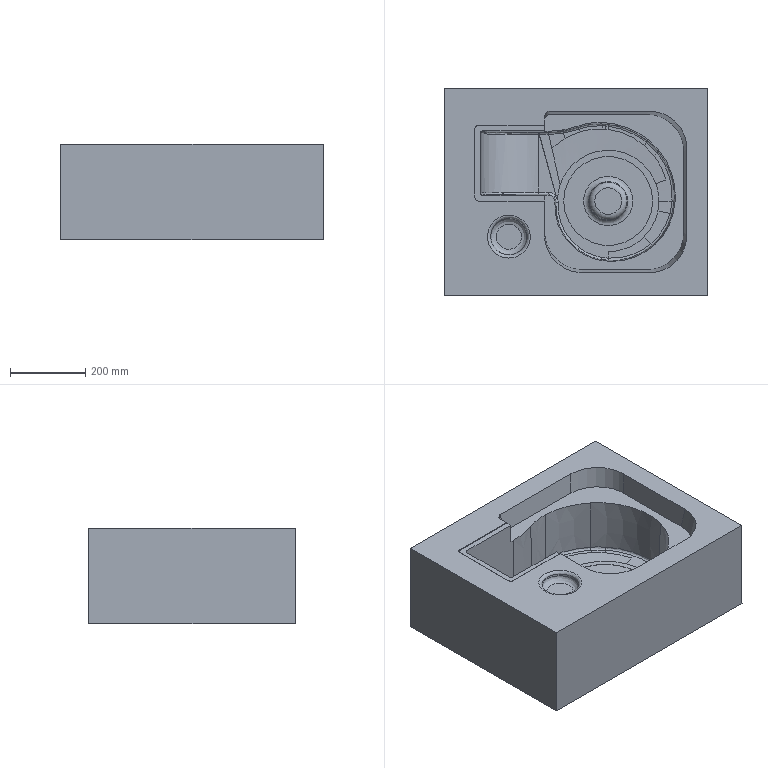NC program | NX | posted with a generic post | part box 700 x 550 x 255 mm
Lines 27406 to 28276 of 43405:
(ZLEVEL_PROFILE , TOOL : 20)
N54798 M6
N54800 G54
N54802 G17 G0 G90 X73.514 Y194.926 S2200 M3
N54804 G43 Z30. H0
N54806 Z0.47
N54808 G94 G1 Z-0.53 F2000.
N54810 G3 X63.514 Y204.926 R10.
N54812 G1 X-68.816
N54814 G3 X-72.579 Y203.186 R4.937
N54816 X-73.824 Y199.761 R5.246
N54818 G1 Y177.182
N54820 G2 X-83.823 Y167.182 R10.
N54822 G1 X-259.307
N54824 G3 X-259.902 Y166.586 R0.595
N54826 G1 Y-13.614
N54828 G3 X-259.307 Y-14.209 R0.595
N54830 G1 X-83.823
N54832 G2 X-73.824 Y-24.209 R10.
N54834 G1 Y-114.065
N54836 G3 X-57.772 Y-165.899 R91.581
N54838 X-18.435 Y-197.973 R90.032
N54840 X16.059 Y-204.926 R89.145
N54842 G1 X195.844
N54844 G3 X233.216 Y-196.836 R89.813
N54846 X279.873 Y-145.675 R88.255
N54848 X284.926 Y-115.894 R90.057
N54850 G1 Y115.894
N54852 G3 X276.844 Y153.199 R89.809
N54854 X226.261 Y199.665 R88.261
N54856 X195.844 Y204.926 R90.036
N54858 G1 X63.514
N54860 G3 X53.514 Y194.926 R10.
N54862 G1 Z0.47
N54864 G0 Z30.
N54866 X73.514 Y194.851
N54868 Z-0.06
N54870 G1 Z-1.06
N54872 G3 X63.514 Y204.851 R10.
N54874 G1 X-68.802
N54876 G3 X-72.812 Y202.812 R4.947
N54878 X-73.819 Y199.722 R5.27
N54880 G1 Y177.177
N54882 G2 X-83.819 Y167.177 R10.
N54884 G1 X-259.307
N54886 G3 X-259.898 Y166.586 R0.591
N54888 G1 Y-13.614
N54890 G3 X-259.307 Y-14.204 R0.591
N54892 G1 X-83.819
N54894 G2 X-73.819 Y-24.204 R10.
N54896 G1 Y-113.991
N54898 G3 X-57.277 Y-166.531 R91.583
N54900 X-17.171 Y-198.417 R90.01
N54902 X16.063 Y-204.851 R89.152
N54904 G1 X195.759
N54906 G3 X232.912 Y-196.866 R89.83
N54908 X280.006 Y-145.002 R88.261
N54910 X284.851 Y-115.816 R90.083
N54912 G1 Y115.816
N54914 G3 X276.995 Y152.627 R89.825
N54916 X224.996 Y200.008 R88.261
N54918 X195.759 Y204.851 R90.09
N54920 G1 X63.514
N54922 G3 X53.514 Y194.851 R10.
N54924 G1 Z-0.06
N54926 G0 Z30.
N54928 X73.514 Y194.777
N54930 Z-0.59
N54932 G1 Z-1.59
N54934 G3 X63.514 Y204.777 R10.
N54936 G1 X-68.787
N54938 G3 X-72.496 Y203.121 R4.929
N54940 X-73.814 Y199.588 R5.239
N54942 G1 Y177.173
N54944 G2 X-83.814 Y167.173 R10.
N54946 G1 X-259.307
N54948 G3 X-259.893 Y166.586 R0.586
N54950 G1 Y-13.614
N54952 G3 X-259.307 Y-14.2 R0.586
N54954 G1 X-83.814
N54956 G2 X-73.814 Y-24.2 R10.
N54958 G1 Y-113.916
N54960 G3 X-58.092 Y-165.267 R91.596
N54962 X-18.435 Y-197.82 R90.043
N54964 X16.068 Y-204.777 R89.148
N54966 G1 X195.683
N54968 G3 X231.952 Y-197.188 R89.86
N54970 X279.892 Y-145.043 R88.268
N54972 X284.777 Y-115.737 R90.098
N54974 G1 Y115.737
N54976 G3 X277.169 Y151.995 R89.847
N54978 X224.996 Y199.908 R88.271
N54980 X195.683 Y204.777 R90.107
N54982 G1 X63.514
N54984 G3 X53.514 Y194.777 R10.
N54986 G1 Z-0.59
N54988 G0 Z30.
N54990 X73.514 Y194.702
N54992 Z-1.12
N54994 G1 Z-2.12
N54996 G3 X63.514 Y204.702 R10.
N54998 G1 X-68.773
N55000 G3 X-72.812 Y202.651 R4.947
N55002 X-73.81 Y199.573 R5.271
N55004 G1 Y177.168
N55006 G2 X-83.81 Y167.168 R10.
N55008 G1 X-259.307
N55010 G3 X-259.889 Y166.586 R0.582
N55012 G1 Y-13.614
N55014 G3 X-259.307 Y-14.195 R0.582
N55016 G1 X-83.81
N55018 G2 X-73.81 Y-24.195 R10.
N55020 G1 Y-113.842
N55022 G3 X-59.291 Y-163.371 R91.639
N55024 X-24.126 Y-195.115 R90.185
N55026 X16.073 Y-204.702 R89.168
N55028 G1 X195.612
N55030 G3 X231.952 Y-197.081 R89.862
N55032 X279.792 Y-145.043 R88.266
N55034 X284.702 Y-115.658 R90.109
N55036 G1 Y115.658
N55038 G3 X276.779 Y152.627 R89.838
N55040 X224.996 Y199.808 R88.268
N55042 X195.612 Y204.702 R90.119
N55044 G1 X63.514
N55046 G3 X53.514 Y194.702 R10.
N55048 G1 Z-1.12
N55050 G0 Z30.
N55052 X-66.304 Y-0.066
N55054 Z-1.817
N55056 G1 Z-2.817
N55058 G3 X-73.804 Y-9.748 R10.
N55060 G1 Y-113.744
N55062 G3 X-58.902 Y-163.861 R91.634
N55064 X-22.861 Y-195.64 R90.139
N55066 X16.079 Y-204.604 R89.171
N55068 G1 X195.523
N55070 G3 X231.952 Y-196.939 R89.888
N55072 X279.659 Y-145.043 R88.267
N55074 X284.604 Y-115.554 R90.12
N55076 G1 Y115.554
N55078 G3 X277.197 Y151.363 R89.907
N55080 X224.996 Y199.675 R88.267
N55082 X195.523 Y204.604 R90.123
N55084 G1 X-68.753
N55086 G3 X-72.534 Y202.892 R4.927
N55088 X-73.796 Y199.647 R5.221
N55090 G1 X-73.804 Y199.394
N55092 Y162.721
N55094 G3 X-66.304 Y153.039 R10.
N55096 G1 Z-1.817
N55098 G0 Z30.
N55100 X-66.297 Y-0.054
N55102 Z-2.515
N55104 G1 Z-3.515
N55106 G3 X-73.797 Y-9.736 R10.
N55108 G1 Y-113.646
N55110 G3 X-59.151 Y-163.371 R91.655
N55112 X-24.126 Y-194.912 R90.167
N55114 X16.085 Y-204.506 R89.164
N55116 G1 X195.436
N55118 G3 X231.319 Y-197.075 R89.879
N55120 X279.076 Y-146.307 R88.246
N55122 X284.506 Y-115.45 R90.068
N55124 G1 Y115.45
N55126 G3 X277.056 Y151.363 R89.895
N55128 X226.261 Y199.092 R88.246
N55130 X195.436 Y204.506 R90.054
N55132 G1 X-68.734
N55134 G3 X-73.138 Y201.922 R4.962
N55136 X-73.797 Y199.246 R5.448
N55138 G1 Y162.709
N55140 G3 X-66.297 Y153.027 R10.
N55142 G1 Z-2.515
N55144 G0 Z30.
N55146 X-66.291 Y-0.042
N55148 Z-3.212
N55150 G1 Z-4.212
N55152 G3 X-73.791 Y-9.724 R10.
N55154 G1 Y-113.548
N55156 G3 X-62.063 Y-158.434 R91.759
N55158 X-28.552 Y-192.415 R90.307
N55160 X16.125 Y-204.408 R89.195
N55162 G1 X195.347
N55164 G3 X231.319 Y-196.935 R89.927
N55166 X279.824 Y-143.779 R88.269
N55168 X284.408 Y-115.349 R90.135
N55170 G1 Y115.349
N55172 G3 X277.458 Y150.099 R89.969
N55174 X225.629 Y199.188 R88.265
N55176 X195.347 Y204.408 R90.116
N55178 G1 X-68.721
N55180 G3 X-73.074 Y201.922 R4.956
N55182 X-73.791 Y199.246 R5.303
N55184 G1 Y162.697
N55186 G3 X-66.291 Y153.014 R10.
N55188 G1 Z-3.212
N55190 G0 Z30.
N55192 X-66.285 Y-0.029
N55194 Z-3.909
N55196 G1 Z-4.909
N55198 G3 X-73.785 Y-9.712 R10.
N55200 G1 Y-113.443
N55202 G3 X-64.592 Y-153.486 R91.802
N55204 X-33.61 Y-189.158 R90.46
N55206 X16.131 Y-204.31 R89.238
N55208 G1 X195.251
N55210 G3 X230.055 Y-197.336 R89.99
N55212 X279.694 Y-143.779 R88.274
N55214 X284.31 Y-115.251 R90.131
N55216 G1 Y115.251
N55218 G3 X277.477 Y149.717 R90.
N55220 X223.732 Y199.709 R88.272
N55222 X195.251 Y204.31 R90.124
N55224 G1 X-68.715
N55226 G3 X-73.01 Y201.922 R4.953
N55228 X-73.785 Y199.097 R5.342
N55230 G1 Y162.685
N55232 G3 X-66.285 Y153.002 R10.
N55234 G1 Z-3.909
N55236 G0 Z30.
N55238 X-66.279 Y-0.017
N55240 Z-4.607
N55242 G1 Z-5.607
N55244 G3 X-73.779 Y-9.7 R10.
N55246 G1 Y-113.352
N55248 G3 X-62.695 Y-157.074 R91.81
N55250 X-33.61 Y-189.056 R90.448
N55252 X16.137 Y-204.212 R89.24
N55254 G1 X195.153
N55256 G3 X227.747 Y-198.13 R90.069
N55258 X278.674 Y-146.307 R88.266
N55260 X284.212 Y-115.153 R90.061
N55262 G1 Y115.153
N55264 G3 X277.7 Y148.835 R90.041
N55266 X226.261 Y198.691 R88.259
N55268 X195.153 Y204.212 R90.067
N55270 G1 X-68.708
N55272 G3 X-73.128 Y201.611 R4.965
N55274 X-73.779 Y199.083 R5.377
N55276 G1 Y162.673
N55278 G3 X-66.279 Y152.99 R10.
N55280 G1 Z-4.607
N55282 G0 Z30.
N55284 X-66.273 Y-0.005
N55286 Z-5.304
N55288 G1 Z-6.304
N55290 G3 X-73.773 Y-9.687 R10.
N55292 G1 Y-113.254
N55294 G3 X-65.487 Y-151.363 R91.834
N55296 X-36.139 Y-187.195 R90.586
N55298 X16.143 Y-204.114 R89.279
N55300 G1 X195.055
N55302 G3 X228.79 Y-197.58 R90.074
N55304 X278.54 Y-146.307 R88.259
N55306 X284.114 Y-115.055 R90.077
N55308 G1 Y115.055
N55310 G3 X277.562 Y148.835 R90.06
N55312 X226.261 Y198.557 R88.259
N55314 X195.055 Y204.114 R90.095
N55316 G1 X-68.702
N55318 G3 X-73.235 Y201.29 R4.967
N55320 X-73.773 Y198.859 R5.378
N55322 G1 Y162.66
N55324 G3 X-66.273 Y152.978 R10.
N55326 G1 Z-5.304
N55328 G0 Z30.
N55330 X-66.267 Y0.007
N55332 Z-6.002
N55334 G1 Z-7.002
N55336 G3 X-73.767 Y-9.675 R10.
N55338 G1 Y-113.156
N55340 G3 X-65.225 Y-151.827 R91.882
N55342 X-36.772 Y-186.632 R90.629
N55344 X11.282 Y-203.883 R89.322
N55346 X16.124 Y-204.016 R88.36
N55348 G1 X194.957
N55350 G3 X227.526 Y-197.944 R90.094
N55352 X279.51 Y-143.147 R88.282
N55354 X284.016 Y-114.957 R90.087
N55356 G1 Y114.957
N55358 G3 X277.477 Y148.706 R90.061
N55360 X225.629 Y198.653 R88.253
N55362 X194.957 Y204.016 R90.075
N55364 G1 X-68.696
N55366 G3 X-73.18 Y201.29 R4.963
N55368 X-73.767 Y198.762 R5.389
N55370 G1 Y162.648
N55372 G3 X-66.267 Y152.966 R10.
N55374 G1 Z-6.002
N55376 G0 Z30.
N55378 X-66.261 Y0.019
N55380 Z-6.699
N55382 G1 Z-7.699
N55384 G3 X-73.761 Y-9.663 R10.
N55386 G1 Y-113.058
N55388 G3 X-65.225 Y-151.716 R91.893
N55390 X-39.933 Y-184.096 R90.792
N55392 X2.43 Y-202.858 R89.489
N55394 X16.155 Y-203.918 R89.473
N55396 G1 X194.858
N55398 G3 X226.893 Y-198.051 R90.155
N55400 X271.294 Y-160.843 R88.274
N55402 G1 X271.668 Y-160.211
N55404 G3 X283.614 Y-122.291 R89.377
N55406 G1 X283.663 Y-121.659
N55408 X283.706 Y-121.027
N55410 G3 X283.918 Y-114.859 R92.451
N55412 G1 Y114.859
N55414 G3 X277.287 Y148.835 R90.066
N55416 X226.893 Y198.051 R88.274
N55418 X194.858 Y203.918 R90.155
N55420 G1 X-68.69
N55422 G3 X-72.18 Y202.532 R4.925
N55424 X-73.717 Y199.394 R5.127
N55426 G1 X-73.757 Y198.762
N55428 X-73.761 Y198.628
N55430 Y162.636
N55432 G3 X-66.261 Y152.954 R10.
N55434 G1 Z-6.699
N55436 G0 Z30.
N55438 X-66.255 Y0.032
N55440 Z-7.396
N55442 G1 Z-8.396
N55444 G3 X-73.755 Y-9.651 R10.
N55446 G1 Y-112.96
N55448 G3 X-65.225 Y-151.605 R91.896
N55450 X-42.462 Y-181.874 R90.811
N55452 X3.695 Y-202.947 R89.473
N55454 X16.161 Y-203.82 R89.56
N55456 G1 X194.76
N55458 G3 X214.248 Y-201.703 R91.154
N55460 X249.151 Y-185.49 R88.843
N55462 G1 X249.656 Y-185.1
N55464 X249.965 Y-184.858
N55466 X250.288 Y-184.604
N55468 X250.76 Y-184.226
N55470 G3 X278.6 Y-145.043 R88.337
N55472 G1 X278.741 Y-144.644
N55474 X278.823 Y-144.411
N55476 X279.039 Y-143.779
N55478 X279.248 Y-143.149
N55480 G3 X283.805 Y-116.017 R89.647
N55482 G1 X283.82 Y-114.761
N55484 Y114.761
N55486 G3 X281.691 Y134.299 R91.142
N55488 X263.03 Y172.219 R88.798
N55490 X223.732 Y199.055 R88.379
N55492 G1 X223.1 Y199.265
N55494 G3 X195.911 Y203.809 R89.856
N55496 G1 X195.279 Y203.813
N55498 X194.76 Y203.82
N55500 X-68.684
N55502 G3 X-72.045 Y202.554 R4.927
N55504 X-73.7 Y199.394 R5.148
N55506 G1 X-73.748 Y198.762
N55508 X-73.755 Y198.636
N55510 Y162.624
N55512 G3 X-66.255 Y152.941 R10.
N55514 G1 Z-7.396
N55516 G0 Z30.
N55518 X-66.249 Y0.044
N55520 Z-8.094
N55522 G1 Z-9.094
N55524 G3 X-73.749 Y-9.639 R10.
N55526 G1 Y-112.862
N55528 G3 X-65.86 Y-150.099 R91.971
N55530 X-44.359 Y-180.075 R90.917
N55532 X-3.892 Y-201.44 R89.598
N55534 X16.167 Y-203.722 R89.268
N55536 G1 X194.663
N55538 G3 X209.822 Y-202.448 R91.941
N55540 X247.127 Y-186.829 R89.06
N55542 X278.465 Y-145.043 R88.311
N55544 G1 X278.69 Y-144.411
N55546 X278.741 Y-144.265
N55548 X278.908 Y-143.779
N55550 X279.136 Y-143.094
N55552 G3 X283.707 Y-115.881 R89.69
N55554 G1 X283.722 Y-114.663
N55556 Y114.663
N55558 G3 X282.544 Y129.243 R91.879
N55560 X266.802 Y167.163 R89.065
N55562 X224.996 Y198.482 R88.321
N55564 G1 X224.364 Y198.707
N55566 X224.204 Y198.762
N55568 X223.732 Y198.924
N55570 X223.018 Y199.161
N55572 G3 X195.932 Y203.706 R89.645
N55574 G1 X194.663 Y203.722
N55576 X-68.678
N55578 G3 X-73.321 Y200.658 R4.99
N55580 X-73.749 Y198.509 R5.584
N55582 G1 Y162.612
N55584 G3 X-66.249 Y152.929 R10.
N55586 G1 Z-8.094
N55588 G0 Z30.
N55590 X-66.243 Y0.056
N55592 Z-8.791
N55594 G1 Z-9.791
N55596 G3 X-73.743 Y-9.627 R10.
N55598 G1 Y-112.764
N55600 G3 X-68.569 Y-143.147 R92.027
N55602 X-43.727 Y-180.55 R90.95
N55604 X-21.597 Y-195.232 R90.06
N55606 X16.173 Y-203.624 R89.173
N55608 G1 X194.565
N55610 G3 X206.028 Y-202.896 R92.448
N55612 X242.701 Y-189.671 R89.154
N55614 X277.127 Y-148.203 R88.221
N55616 X283.615 Y-115.339 R89.771
N55618 G1 X283.624 Y-114.565
N55620 Y114.565
N55622 G3 X282.53 Y128.611 R91.938
N55624 X268.402 Y164.635 R89.035
N55626 X224.996 Y198.348 R88.273
N55628 X195.911 Y203.61 R89.847
N55630 G1 X195.279 Y203.615
N55632 X194.565 Y203.624
N55634 X-68.672
N55636 G3 X-73.273 Y200.658 R4.985
N55638 X-73.743 Y198.354 R5.536
N55640 G1 Y162.6
N55642 G3 X-66.243 Y152.917 R10.
N55644 G1 Z-8.791
N55646 G0 Z30.
N55648 X-66.237 Y0.068
N55650 Z-9.488
N55652 G1 Z-10.488
N55654 G3 X-73.737 Y-9.614 R10.
N55656 G1 Y-112.666
N55658 G3 X-63.958 Y-153.891 R91.845
N55660 X-38.443 Y-184.858 R90.642
N55662 X6.224 Y-202.97 R89.408
N55664 X16.11 Y-203.526 R88.22
N55666 G1 X194.467
N55668 G3 X203.499 Y-203.074 R92.902
N55670 X238.275 Y-192.161 R89.333
N55672 X276.99 Y-148.203 R88.24
N55674 X283.516 Y-115.339 R89.803
N55676 G1 X283.526 Y-114.467
N55678 Y114.467
N55680 G3 X282.316 Y129.243 R91.942
N55682 X269.487 Y162.739 R89.141
N55684 X225.629 Y197.984 R88.259
N55686 X195.279 Y203.516 R89.8
N55688 G1 X194.467 Y203.526
N55690 X-68.666
N55692 G3 X-73.22 Y200.658 R4.98
N55694 X-73.737 Y198.354 R5.433
N55696 G1 Y162.587
N55698 G3 X-66.237 Y152.905 R10.
N55700 G1 Z-9.488
N55702 G0 Z30.
N55704 X-66.231 Y0.08
N55706 Z-10.186
N55708 G1 Z-11.186
N55710 G3 X-73.731 Y-9.602 R10.
N55712 G1 Y-112.568
N55714 G3 X-71.12 Y-134.299 R92.428
N55716 X-51.314 Y-172.616 R91.202
N55718 X-20.332 Y-195.61 R89.944
N55720 X16.185 Y-203.428 R89.19
N55722 G1 X194.369
N55724 G3 X208.557 Y-202.312 R92.036
N55726 X240.171 Y-190.911 R89.145
N55728 X278.109 Y-144.917 R88.257
N55730 X283.379 Y-117.235 R89.776
N55732 X283.428 Y-114.369 R98.294
N55734 G1 Y114.369
N55736 G3 X278.514 Y143.779 R90.279
N55738 X255.715 Y179.171 R88.469
N55740 X221.089 Y199.394 R88.56
N55742 G1 X220.57 Y199.55
N55744 G3 X195.279 Y203.417 R89.888
N55746 G1 X194.369 Y203.428
N55748 X-68.66
N55750 G3 X-72.812 Y201.258 R4.962
N55752 X-73.724 Y198.353 R5.238
N55754 G1 X-73.731 Y198.13
N55756 Y162.575
N55758 G3 X-66.231 Y152.893 R10.
N55760 G1 Z-10.186
N55762 G0 Z30.
N55764 X-66.224 Y0.092
N55766 Z-10.883
N55768 G1 Z-11.883
N55770 G3 X-73.724 Y-9.59 R10.
N55772 G1 Y-112.47
N55774 G3 X-71.802 Y-131.139 R92.406
N55776 X-50.682 Y-173.229 R91.199
N55778 X-18.435 Y-196.336 R89.923
N55780 X16.192 Y-203.33 R89.19
N55782 G1 X194.271
N55784 G3 X221.203 Y-199.231 R90.494
N55786 X252.817 Y-181.61 R88.667
N55788 X279.373 Y-140.734 R88.424
N55790 X283.318 Y-115.339 R89.927
N55792 G1 X283.33 Y-114.271
N55794 Y114.271
N55796 G3 X282.19 Y128.611 R92.075
N55798 X269.257 Y162.596 R89.143
N55800 X228.108 Y196.753 R88.266
N55802 X199.008 Y203.203 R89.69
N55804 X194.271 Y203.33 R97.119
N55806 G1 X-68.654
N55808 G3 X-72.297 Y201.787 R4.943
N55810 X-73.709 Y198.468 R5.173
N55812 G1 X-73.724 Y198.13
N55814 Y162.563
N55816 G3 X-66.224 Y152.881 R10.
N55818 G1 Z-10.883
N55820 G0 Z30.
N55822 X-66.218 Y0.105
N55824 Z-11.581
N55826 G1 Z-12.581
N55828 G3 X-73.718 Y-9.578 R10.
N55830 G1 Y-112.372
N55832 G3 X-70.401 Y-136.827 R92.327
N55834 X-51.314 Y-172.406 R91.211
N55836 X-20.964 Y-195.122 R89.997
N55838 X16.198 Y-203.232 R89.161
N55840 G1 X194.173
N55842 G3 X202.234 Y-202.871 R94.374
N55844 X237.642 Y-192.054 R89.356
N55846 X275.774 Y-150.099 R88.17
N55848 X283.219 Y-115.339 R89.642
N55850 G1 X283.224 Y-114.707
N55852 X283.232 Y-114.172
N55854 Y114.172
N55856 G3 X283.056 Y119.763 R98.131
N55858 X272.032 Y157.683 R89.401
N55860 X230.495 Y195.602 R88.212
N55862 X195.279 Y203.22 R89.705
N55864 G1 X194.173 Y203.232
N55866 X-68.648
N55868 G3 X-72.832 Y201.013 R4.963
N55870 X-73.702 Y198.343 R5.248
N55872 G1 X-73.718 Y197.975
N55874 Y162.551
N55876 G3 X-66.218 Y152.868 R10.
N55878 G1 Z-11.581
N55880 G0 Z30.
N55882 X-66.212 Y0.117
N55884 Z-12.278
N55886 G1 Z-13.278
N55888 G3 X-73.712 Y-9.566 R10.
N55890 G1 Y-112.274
N55892 G3 X-72.18 Y-128.971 R93.023
N55894 X-56.848 Y-165.267 R91.413
N55896 X-23.493 Y-193.814 R90.104
N55898 X16.204 Y-203.134 R89.202
N55900 G1 X194.075
N55902 G3 X200.337 Y-202.914 R97.029
N55904 X235.462 Y-193.074 R89.445
N55906 G1 X235.745 Y-192.927
N55908 X236.378 Y-192.586
N55910 X237.01 Y-192.248
N55912 X237.642 Y-191.902
N55914 X237.808 Y-191.81
N55916 X238.275 Y-191.546
N55918 X238.911 Y-191.178
N55920 X239.539 Y-190.816
N55922 X239.997 Y-190.546
N55924 X240.171 Y-190.442
N55926 X240.804 Y-190.053
N55928 X241.436 Y-189.666
N55930 X242.068 Y-189.271
N55932 X242.701 Y-188.863
N55934 X243.024 Y-188.65
N55936 X243.333 Y-188.449
N55938 X243.986 Y-188.018
N55940 X244.597 Y-187.605
N55942 X244.91 Y-187.386
N55944 X245.23 Y-187.162
N55946 X245.862 Y-186.724
N55948 X246.494 Y-186.272
N55950 X246.698 Y-186.122
N55952 X247.127 Y-185.803
N55954 X247.551 Y-185.49
N55956 X247.759 Y-185.337
N55958 X248.394 Y-184.858
N55960 X249.023 Y-184.372
N55962 X249.209 Y-184.226
N55964 X249.656 Y-183.875
N55966 X250.007 Y-183.594
N55968 X250.288 Y-183.368
N55970 X250.786 Y-182.962
N55972 X250.92 Y-182.852
N55974 X251.553 Y-182.328
N55976 X252.291 Y-181.698
N55978 X252.817 Y-181.242
N55980 X253.017 Y-181.066
N55982 X253.45 Y-180.686
N55984 G3 X277.477 Y-145.551 R88.386
N55986 G1 X277.661 Y-145.043
N55988 G3 X283.073 Y-117.235 R89.503
N55990 X283.134 Y-114.075 R101.206
N55992 G1 Y114.075
N55994 G3 X283.073 Y117.235 R101.206
N55996 X274.483 Y152.627 R89.559
N55998 X231.581 Y194.97 R88.202
N56000 X199.705 Y202.956 R89.501
N56002 X194.075 Y203.134 R98.01
N56004 G1 X-68.697
N56006 G3 X-72.876 Y200.835 R4.948
N56008 G1 X-72.91 Y200.781
N56010 G3 X-73.693 Y198.335 R5.082
N56012 G1 X-73.712 Y197.975
N56014 Y162.539
N56016 G3 X-66.212 Y152.856 R10.
N56018 G1 Z-12.278
N56020 G0 Z30.
N56022 X-66.206 Y0.129
N56024 Z-12.975
N56026 G1 Z-13.975
N56028 G3 X-73.706 Y-9.554 R10.
N56030 G1 Y-112.176
N56032 G3 X-73.071 Y-122.923 R94.608
N56034 X-62.695 Y-155.762 R91.631
N56036 X-40.565 Y-182.652 R90.721
N56038 X-5.157 Y-200.441 R89.591
N56040 X16.21 Y-203.036 R89.191
N56042 G1 X193.977
N56044 G3 X199.118 Y-202.886 R98.516
N56046 X232.584 Y-194.359 R89.499
N56048 X267.844 Y-164.003 R88.271
N56050 X282.043 Y-127.347 R89.025
N56052 X283.021 Y-115.339 R89.525
N56054 G1 X283.036 Y-113.977
N56056 Y113.977
N56058 G3 X282.894 Y118.951 R99.521
N56060 X274.339 Y152.627 R89.512
N56062 X248.391 Y184.687 R88.318
N56064 X212.983 Y201.019 R88.794
N56066 G1 X212.351 Y201.152
N56068 X211.718 Y201.287
N56070 X211.086 Y201.409
N56072 X210.454 Y201.525
N56074 G3 X195.279 Y203.022 R89.716
N56076 G1 X193.977 Y203.036
N56078 X-68.636
N56080 G3 X-73.254 Y200.026 R4.992
N56082 X-73.706 Y197.819 R5.544
N56084 G1 Y162.527
N56086 G3 X-66.206 Y152.844 R10.
N56088 G1 Z-12.975
N56090 G0 Z30.
N56092 X-66.2 Y0.141
N56094 Z-13.673
N56096 G1 Z-14.673
N56098 G3 X-73.7 Y-9.541 R10.
N56100 G1 Y-112.078
N56102 G3 X-73.196 Y-121.659 R96.158
N56104 X-62.621 Y-155.787 R91.656
N56106 X-44.359 Y-179.246 R90.768
N56108 X-16.538 Y-196.707 R89.82
N56110 X16.216 Y-202.938 R89.186
N56112 G1 X193.879
N56114 G3 X200.337 Y-202.705 R98.064
N56116 X232.584 Y-194.214 R89.525
N56118 X265.906 Y-166.531 R88.28
N56120 X279.641 Y-138.091 R88.809
N56122 X282.922 Y-115.339 R90.149
N56124 G1 X282.938 Y-113.879
N56126 Y113.879
N56128 G3 X282.701 Y120.395 R98.537
N56130 X274.194 Y152.627 R89.562
N56132 X249.566 Y183.594 R88.318
N56134 X215.512 Y200.316 R88.716
N56136 X195.279 Y202.923 R90.135
N56138 G1 X193.879 Y202.938
N56140 X-68.629
N56142 G3 X-72.812 Y200.72 R4.966
N56144 X-73.691 Y197.974 R5.242
N56146 G1 X-73.7 Y197.658
N56148 Y162.514
N56150 G3 X-66.2 Y152.832 R10.
N56152 G1 Z-13.673
N56154 G0 Z30.
N56156 X-66.194 Y0.153
N56158 Z-14.37
N56160 G1 Z-15.37
N56162 G3 X-73.694 Y-9.529 R10.
N56164 G1 Y-111.98
N56166 G3 X-73.242 Y-121.027 R96.284
N56168 X-62.561 Y-155.787 R91.563
N56170 X-36.139 Y-185.863 R90.535
N56172 X-3.892 Y-200.545 R89.583
N56174 X16.222 Y-202.84 R89.219
N56176 G1 X193.781
N56178 G3 X200.337 Y-202.6 R97.939
N56180 X227.526 Y-196.299 R89.589
N56182 X275.212 Y-150.099 R88.232
N56184 X282.597 Y-120.395 R89.636
N56186 X282.84 Y-113.781 R97.885
N56188 G1 Y113.781
N56190 G3 X282.597 Y120.395 R97.885
N56192 X275.212 Y150.099 R89.636
N56194 X237.01 Y191.795 R88.234
N56196 G1 X236.378 Y192.134
N56198 X235.745 Y192.478
N56200 X235.113 Y192.809
N56202 G3 X204.763 Y202.169 R89.256
N56204 G1 X204.131 Y202.249
N56206 X203.499 Y202.319
N56208 X202.717 Y202.397
N56210 G3 X194.88 Y202.828 R88.919
N56212 G1 X193.781 Y202.84
N56214 X-68.623
N56216 G3 X-72.688 Y200.791 R4.969
N56218 X-73.686 Y197.818 R5.23
N56220 G1 X-73.694 Y197.658
N56222 Y162.502
N56224 G3 X-66.194 Y152.82 R10.
N56226 G1 Z-14.37
N56228 G0 Z30.
N56230 X-66.188 Y0.165
N56232 Z-15.067
N56234 G1 Z-16.067
N56236 G3 X-73.688 Y-9.517 R10.
N56238 G1 Y-111.882
N56240 G3 X-73.226 Y-121.027 R96.461
N56242 X-62.843 Y-155.155 R91.571
N56244 X-36.139 Y-185.761 R90.539
N56246 X-5.157 Y-200.143 R89.618
N56248 X16.228 Y-202.742 R89.176
N56250 G1 X193.683
N56252 G3 X200.337 Y-202.495 R97.419
N56254 X230.055 Y-195.091 R89.642
N56256 X261.037 Y-172.213 R88.349
N56258 G1 X261.669 Y-171.473
N56260 X262.106 Y-170.955
N56262 X262.323 Y-170.693
N56264 G3 X278.992 Y-139.462 R88.596
N56266 G1 X279.212 Y-138.723
N56268 X279.392 Y-138.091
N56270 X279.561 Y-137.459
N56272 G3 X282.729 Y-114.707 R89.643
N56274 G1 X282.742 Y-113.683
N56276 Y113.683
N56278 G3 X282.492 Y120.395 R96.979
N56280 X275.071 Y150.099 R89.678
N56282 X251.439 Y181.698 R88.344
N56284 G1 X250.92 Y182.135
N56286 X250.684 Y182.33
N56288 X250.288 Y182.658
N56290 X249.913 Y182.962
N56292 X249.656 Y183.169
N56294 X249.124 Y183.594
N56296 G3 X215.512 Y200.073 R88.794
N56298 G1 X214.88 Y200.224
N56300 G3 X194.647 Y202.729 R89.574
N56302 G1 X193.683 Y202.742
N56304 X-68.617
N56306 G3 X-72.812 Y200.505 R4.968
N56308 X-73.674 Y197.817 R5.24
N56310 G1 X-73.688 Y197.498
N56312 Y162.49
N56314 G3 X-66.188 Y152.808 R10.
N56316 G1 Z-15.067
N56318 G0 Z30.
N56320 X-66.182 Y0.178
N56322 Z-15.765
N56324 G1 Z-16.765
N56326 G3 X-73.682 Y-9.505 R10.
N56328 G1 Y-111.784
N56330 G3 X-70.878 Y-134.299 R92.449
N56332 X-62.695 Y-155.324 R91.828
N56334 X-54.58 Y-167.795 R91.719
N56336 X-34.242 Y-186.994 R90.345
N56338 X-27.919 Y-190.951 R91.757
N56340 X8.753 Y-202.331 R89.352
N56342 X16.17 Y-202.644 R88.042
N56344 G1 X193.584
N56346 G3 X200.337 Y-202.39 R96.63
N56348 X228.79 Y-195.498 R89.659
N56350 X263.471 Y-169.059 R88.34
N56352 X281.165 Y-129.875 R88.813
N56354 X282.63 Y-114.707 R89.174
N56356 G1 X282.637 Y-114.075
N56358 X282.644 Y-113.585
N56360 Y113.585
N56362 G3 X282.283 Y121.659 R95.015
N56364 X273.683 Y152.785 R89.589
N56366 X263.471 Y169.059 R89.178
N56368 X224.996 Y197.008 R88.331
N56370 G1 X224.364 Y197.239
N56372 X223.732 Y197.473
N56374 G3 X197.808 Y202.544 R90.183
N56376 G1 X197.176 Y202.566
N56378 X196.543 Y202.593
N56380 G3 X193.584 Y202.644 R122.036
N56382 G1 X-68.611
N56384 G3 X-73.12 Y199.866 R4.989
N56386 X-73.664 Y197.782 R5.311
N56388 G1 X-73.682 Y197.425
N56390 Y162.478
N56392 G3 X-66.182 Y152.795 R10.
N56394 G1 Z-15.765
N56396 G0 Z30.
N56398 X-66.176 Y0.19
N56400 Z-16.462
N56402 G1 Z-17.462
N56404 G3 X-73.676 Y-9.493 R10.
N56406 G1 Y-111.686
N56408 G3 X-73.314 Y-119.763 R96.042
N56410 X-63.718 Y-153.259 R91.575
N56412 X-44.359 Y-178.83 R90.712
N56414 X-23.493 Y-193.207 R90.023
N56416 X8.753 Y-202.232 R89.369
N56418 X16.173 Y-202.546 R87.987
N56420 G1 X193.486
N56422 G3 X201.602 Y-202.181 R94.83
N56424 X232.433 Y-193.706 R89.532
N56426 X258.37 Y-174.747 R88.437
N56428 X279.373 Y-137.233 R88.539
N56430 G1 X279.484 Y-136.827
N56432 G3 X282.525 Y-115.339 R90.173
N56434 G1 X282.535 Y-114.283
N56436 X282.538 Y-114.075
N56438 X282.546 Y-113.487
N56440 Y113.487
N56442 G3 X282.488 Y116.603 R106.184
N56444 X275.868 Y147.571 R89.776
N56446 X254.714 Y178.401 R88.417
N56448 X222.044 Y197.916 R88.425
N56450 G1 X221.835 Y197.986
N56452 X221.408 Y198.13
N56454 X221.203 Y198.199
N56456 X220.57 Y198.399
N56458 X219.938 Y198.591
N56460 G3 X199.073 Y202.372 R89.715
N56462 X193.486 Y202.546 R96.891
N56464 G1 X-68.605
N56466 G3 X-73.489 Y198.762 R5.005
N56468 X-73.676 Y197.351 R6.112
N56470 G1 Y162.466
N56472 G3 X-66.176 Y152.783 R10.
N56474 G1 Z-16.462
N56476 G0 Z30.
N56478 X-66.17 Y0.202
N56480 Z-17.159
N56482 G1 Z-18.159
N56484 G3 X-73.67 Y-9.481 R10.
N56486 G1 Y-111.588
N56488 G3 X-73.356 Y-119.131 R99.949
N56490 X-63.96 Y-152.675 R91.771
N56492 X-52.897 Y-169.691 R91.178
N56494 X-30.392 Y-189.282 R89.992
N56496 X11.282 Y-202.31 R89.221
N56498 X16.213 Y-202.448 R88.446
N56500 G1 X193.389
N56502 G3 X202.866 Y-201.952 R93.837
N56504 X226.261 Y-196.256 R89.846
N56506 X255.688 Y-177.275 R88.47
N56508 X270.806 Y-157.683 R88.263
N56510 X281.721 Y-124.819 R89.157
N56512 X282.429 Y-114.789 R87.805
N56514 G1 X282.448 Y-113.389
N56516 Y113.389
N56518 G3 X281.946 Y122.923 R94.987
N56520 X274.647 Y150.099 R89.652
N56522 X270.075 Y158.947 R90.032
N56524 X265.972 Y165.267 R90.27
N56526 X231.952 Y193.79 R88.208
N56528 G1 X231.319 Y194.084
N56530 X230.781 Y194.338
N56532 G3 X204.131 Y201.809 R89.542